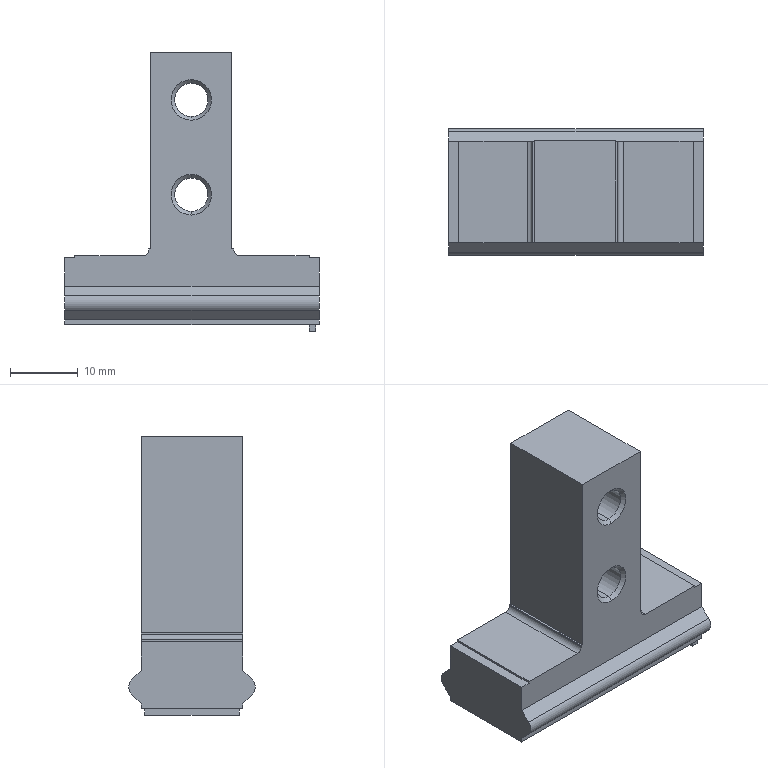Part | SolidWorks | features BaseBody 1 | 1 solid | 45 faces | box 37.6 x 18.7 x 41.2 mm | volume 11010 mm3 | plane 29 | cone 8 | cylinder 8 | commonest cylinder face diameters 4.917 x4 1.6 x2 3 x2
STEP:
#1=CARTESIAN_POINT('',(-30.,-6.958,35.659));
#2=VERTEX_POINT('',#1);
#3=CARTESIAN_POINT('',(-30.,-6.958,30.741));
#4=VERTEX_POINT('',#3);
#5=CARTESIAN_POINT('',(-30.,-6.958,33.2));
#6=DIRECTION('',(0.,-1.,0.));
#7=DIRECTION('',(0.,0.,-1.));
#8=AXIS2_PLACEMENT_3D('',#5,#6,#7);
#9=CIRCLE('',#8,2.459);
#10=EDGE_CURVE('',#2,#4,#9,.T.);
#11=ORIENTED_EDGE('',*,*,#10,.F.);
#12=CARTESIAN_POINT('',(-30.,-7.5,36.2));
#13=VERTEX_POINT('',#12);
#14=CARTESIAN_POINT('',(-30.,-6.958,35.659));
#15=DIRECTION('',(0.,-0.7071,0.7071));
#16=VECTOR('',#15,1000.);
#17=LINE('',#14,#16);
#18=EDGE_CURVE('',#2,#13,#17,.T.);
#19=ORIENTED_EDGE('',*,*,#18,.T.);
#20=CARTESIAN_POINT('',(-30.,-7.5,30.2));
#21=VERTEX_POINT('',#20);
#22=CARTESIAN_POINT('',(-30.,-7.5,33.2));
#23=DIRECTION('',(0.,-1.,0.));
#24=DIRECTION('',(0.,0.,-1.));
#25=AXIS2_PLACEMENT_3D('',#22,#23,#24);
#26=CIRCLE('',#25,3.);
#27=EDGE_CURVE('',#13,#21,#26,.T.);
#28=ORIENTED_EDGE('',*,*,#27,.T.);
#29=CARTESIAN_POINT('',(-30.,-6.958,30.741));
#30=DIRECTION('',(0.,-0.7071,-0.7071));
#31=VECTOR('',#30,1000.);
#32=LINE('',#29,#31);
#33=EDGE_CURVE('',#4,#21,#32,.T.);
#34=ORIENTED_EDGE('',*,*,#33,.F.);
#35=EDGE_LOOP('',(#11,#19,#28,#34));
#36=FACE_OUTER_BOUND('',#35,.T.);
#37=CARTESIAN_POINT('',(-30.,-6.958,33.2));
#38=DIRECTION('',(0.,-1.,0.));
#39=DIRECTION('',(0.,0.,-1.));
#40=AXIS2_PLACEMENT_3D('',#37,#38,#39);
#41=CONICAL_SURFACE('',#40,2.459,0.7854);
#42=ADVANCED_FACE('',(#36),#41,.F.);
#43=CARTESIAN_POINT('',(-30.,-6.958,21.659));
#44=VERTEX_POINT('',#43);
#45=CARTESIAN_POINT('',(-30.,-6.958,16.741));
#46=VERTEX_POINT('',#45);
#47=CARTESIAN_POINT('',(-30.,-6.958,19.2));
#48=DIRECTION('',(0.,-1.,0.));
#49=DIRECTION('',(0.,0.,-1.));
#50=AXIS2_PLACEMENT_3D('',#47,#48,#49);
#51=CIRCLE('',#50,2.459);
#52=EDGE_CURVE('',#44,#46,#51,.T.);
#53=ORIENTED_EDGE('',*,*,#52,.F.);
#54=CARTESIAN_POINT('',(-30.,-7.5,22.2));
#55=VERTEX_POINT('',#54);
#56=CARTESIAN_POINT('',(-30.,-6.958,21.658));
#57=DIRECTION('',(0.,-0.7071,0.7071));
#58=VECTOR('',#57,1000.);
#59=LINE('',#56,#58);
#60=EDGE_CURVE('',#44,#55,#59,.T.);
#61=ORIENTED_EDGE('',*,*,#60,.T.);
#62=CARTESIAN_POINT('',(-30.,-7.5,16.2));
#63=VERTEX_POINT('',#62);
#64=CARTESIAN_POINT('',(-30.,-7.5,19.2));
#65=DIRECTION('',(0.,-1.,0.));
#66=DIRECTION('',(0.,0.,-1.));
#67=AXIS2_PLACEMENT_3D('',#64,#65,#66);
#68=CIRCLE('',#67,3.);
#69=EDGE_CURVE('',#55,#63,#68,.T.);
#70=ORIENTED_EDGE('',*,*,#69,.T.);
#71=CARTESIAN_POINT('',(-30.,-6.958,16.741));
#72=DIRECTION('',(0.,-0.7071,-0.7071));
#73=VECTOR('',#72,1000.);
#74=LINE('',#71,#73);
#75=EDGE_CURVE('',#46,#63,#74,.T.);
#76=ORIENTED_EDGE('',*,*,#75,.F.);
#77=EDGE_LOOP('',(#53,#61,#70,#76));
#78=FACE_OUTER_BOUND('',#77,.T.);
#79=CARTESIAN_POINT('',(-30.,-6.958,19.2));
#80=DIRECTION('',(0.,-1.,0.));
#81=DIRECTION('',(0.,0.,-1.));
#82=AXIS2_PLACEMENT_3D('',#79,#80,#81);
#83=CONICAL_SURFACE('',#82,2.458,0.7854);
#84=ADVANCED_FACE('',(#78),#83,.F.);
#85=CARTESIAN_POINT('',(-30.,6.958,35.659));
#86=VERTEX_POINT('',#85);
#87=CARTESIAN_POINT('',(-30.,6.958,30.741));
#88=VERTEX_POINT('',#87);
#89=CARTESIAN_POINT('',(-30.,6.958,33.2));
#90=DIRECTION('',(0.,-1.,0.));
#91=DIRECTION('',(0.,0.,-1.));
#92=AXIS2_PLACEMENT_3D('',#89,#90,#91);
#93=CIRCLE('',#92,2.459);
#94=EDGE_CURVE('',#86,#88,#93,.T.);
#95=ORIENTED_EDGE('',*,*,#94,.F.);
#96=CARTESIAN_POINT('',(-30.,-7.5,35.659));
#97=DIRECTION('',(0.,-1.,0.));
#98=VECTOR('',#97,1000.);
#99=LINE('',#96,#98);
#100=EDGE_CURVE('',#86,#2,#99,.T.);
#101=ORIENTED_EDGE('',*,*,#100,.T.);
#102=ORIENTED_EDGE('',*,*,#10,.T.);
#103=CARTESIAN_POINT('',(-30.,-7.5,30.741));
#104=DIRECTION('',(0.,-1.,0.));
#105=VECTOR('',#104,1000.);
#106=LINE('',#103,#105);
#107=EDGE_CURVE('',#88,#4,#106,.T.);
#108=ORIENTED_EDGE('',*,*,#107,.F.);
#109=EDGE_LOOP('',(#95,#101,#102,#108));
#110=FACE_OUTER_BOUND('',#109,.T.);
#111=CARTESIAN_POINT('',(-30.,-7.5,33.2));
#112=DIRECTION('',(0.,-1.,0.));
#113=DIRECTION('',(0.,0.,-1.));
#114=AXIS2_PLACEMENT_3D('',#111,#112,#113);
#115=CYLINDRICAL_SURFACE('',#114,2.459);
#116=ADVANCED_FACE('',(#110),#115,.F.);
#117=CARTESIAN_POINT('',(-30.,6.958,21.659));
#118=VERTEX_POINT('',#117);
#119=CARTESIAN_POINT('',(-30.,6.958,16.741));
#120=VERTEX_POINT('',#119);
#121=CARTESIAN_POINT('',(-30.,6.958,19.2));
#122=DIRECTION('',(0.,-1.,0.));
#123=DIRECTION('',(0.,0.,-1.));
#124=AXIS2_PLACEMENT_3D('',#121,#122,#123);
#125=CIRCLE('',#124,2.459);
#126=EDGE_CURVE('',#118,#120,#125,.T.);
#127=ORIENTED_EDGE('',*,*,#126,.F.);
#128=CARTESIAN_POINT('',(-30.,-7.5,21.658));
#129=DIRECTION('',(0.,-1.,0.));
#130=VECTOR('',#129,1000.);
#131=LINE('',#128,#130);
#132=EDGE_CURVE('',#118,#44,#131,.T.);
#133=ORIENTED_EDGE('',*,*,#132,.T.);
#134=ORIENTED_EDGE('',*,*,#52,.T.);
#135=CARTESIAN_POINT('',(-30.,-7.5,16.741));
#136=DIRECTION('',(0.,-1.,0.));
#137=VECTOR('',#136,1000.);
#138=LINE('',#135,#137);
#139=EDGE_CURVE('',#120,#46,#138,.T.);
#140=ORIENTED_EDGE('',*,*,#139,.F.);
#141=EDGE_LOOP('',(#127,#133,#134,#140));
#142=FACE_OUTER_BOUND('',#141,.T.);
#143=CARTESIAN_POINT('',(-30.,-7.5,19.2));
#144=DIRECTION('',(0.,-1.,0.));
#145=DIRECTION('',(0.,0.,-1.));
#146=AXIS2_PLACEMENT_3D('',#143,#144,#145);
#147=CYLINDRICAL_SURFACE('',#146,2.458);
#148=ADVANCED_FACE('',(#142),#147,.F.);
#149=ORIENTED_EDGE('',*,*,#94,.T.);
#150=CARTESIAN_POINT('',(-30.,7.5,30.2));
#151=VERTEX_POINT('',#150);
#152=CARTESIAN_POINT('',(-30.,7.5,30.2));
#153=DIRECTION('',(0.,0.7071,-0.7071));
#154=VECTOR('',#153,1000.);
#155=LINE('',#152,#154);
#156=EDGE_CURVE('',#88,#151,#155,.T.);
#157=ORIENTED_EDGE('',*,*,#156,.T.);
#158=CARTESIAN_POINT('',(-30.,7.5,36.2));
#159=VERTEX_POINT('',#158);
#160=CARTESIAN_POINT('',(-30.,7.5,33.2));
#161=DIRECTION('',(0.,-1.,0.));
#162=DIRECTION('',(0.,0.,-1.));
#163=AXIS2_PLACEMENT_3D('',#160,#161,#162);
#164=CIRCLE('',#163,3.);
#165=EDGE_CURVE('',#159,#151,#164,.T.);
#166=ORIENTED_EDGE('',*,*,#165,.F.);
#167=CARTESIAN_POINT('',(-30.,7.5,36.2));
#168=DIRECTION('',(0.,0.7071,0.7071));
#169=VECTOR('',#168,1000.);
#170=LINE('',#167,#169);
#171=EDGE_CURVE('',#86,#159,#170,.T.);
#172=ORIENTED_EDGE('',*,*,#171,.F.);
#173=EDGE_LOOP('',(#149,#157,#166,#172));
#174=FACE_OUTER_BOUND('',#173,.T.);
#175=CARTESIAN_POINT('',(-30.,7.5,33.2));
#176=DIRECTION('',(0.,1.,0.));
#177=DIRECTION('',(0.,0.,1.));
#178=AXIS2_PLACEMENT_3D('',#175,#176,#177);
#179=CONICAL_SURFACE('',#178,3.,0.7854);
#180=ADVANCED_FACE('',(#174),#179,.F.);
#181=ORIENTED_EDGE('',*,*,#126,.T.);
#182=CARTESIAN_POINT('',(-30.,7.5,16.2));
#183=VERTEX_POINT('',#182);
#184=CARTESIAN_POINT('',(-30.,7.5,16.2));
#185=DIRECTION('',(0.,0.7071,-0.7071));
#186=VECTOR('',#185,1000.);
#187=LINE('',#184,#186);
#188=EDGE_CURVE('',#120,#183,#187,.T.);
#189=ORIENTED_EDGE('',*,*,#188,.T.);
#190=CARTESIAN_POINT('',(-30.,7.5,22.2));
#191=VERTEX_POINT('',#190);
#192=CARTESIAN_POINT('',(-30.,7.5,19.2));
#193=DIRECTION('',(0.,-1.,0.));
#194=DIRECTION('',(0.,0.,-1.));
#195=AXIS2_PLACEMENT_3D('',#192,#193,#194);
#196=CIRCLE('',#195,3.);
#197=EDGE_CURVE('',#191,#183,#196,.T.);
#198=ORIENTED_EDGE('',*,*,#197,.F.);
#199=CARTESIAN_POINT('',(-30.,7.5,22.2));
#200=DIRECTION('',(0.,0.7071,0.7071));
#201=VECTOR('',#200,1000.);
#202=LINE('',#199,#201);
#203=EDGE_CURVE('',#118,#191,#202,.T.);
#204=ORIENTED_EDGE('',*,*,#203,.F.);
#205=EDGE_LOOP('',(#181,#189,#198,#204));
#206=FACE_OUTER_BOUND('',#205,.T.);
#207=CARTESIAN_POINT('',(-30.,7.5,19.2));
#208=DIRECTION('',(0.,1.,0.));
#209=DIRECTION('',(0.,0.,1.));
#210=AXIS2_PLACEMENT_3D('',#207,#208,#209);
#211=CONICAL_SURFACE('',#210,3.,0.7854);
#212=ADVANCED_FACE('',(#206),#211,.F.);
#213=CARTESIAN_POINT('',(-47.2,7.5,9.9));
#214=VERTEX_POINT('',#213);
#215=CARTESIAN_POINT('',(-48.7,7.5,9.9));
#216=VERTEX_POINT('',#215);
#217=CARTESIAN_POINT('',(-47.2,7.5,9.9));
#218=DIRECTION('',(-1.,0.,0.));
#219=VECTOR('',#218,1000.);
#220=LINE('',#217,#219);
#221=EDGE_CURVE('',#214,#216,#220,.T.);
#222=ORIENTED_EDGE('',*,*,#221,.F.);
#223=CARTESIAN_POINT('',(-47.2,7.5,10.2));
#224=VERTEX_POINT('',#223);
#225=CARTESIAN_POINT('',(-47.2,7.5,9.9));
#226=DIRECTION('',(0.,0.,1.));
#227=VECTOR('',#226,1000.);
#228=LINE('',#225,#227);
#229=EDGE_CURVE('',#214,#224,#228,.T.);
#230=ORIENTED_EDGE('',*,*,#229,.T.);
#231=CARTESIAN_POINT('',(-37.1,7.5,10.2));
#232=VERTEX_POINT('',#231);
#233=CARTESIAN_POINT('',(-47.2,7.5,10.2));
#234=DIRECTION('',(1.,0.,0.));
#235=VECTOR('',#234,1000.);
#236=LINE('',#233,#235);
#237=EDGE_CURVE('',#224,#232,#236,.T.);
#238=ORIENTED_EDGE('',*,*,#237,.T.);
#239=CARTESIAN_POINT('',(-36.3,7.5,11.));
#240=VERTEX_POINT('',#239);
#241=CARTESIAN_POINT('',(-37.1,7.5,11.));
#242=DIRECTION('',(0.,1.,0.));
#243=DIRECTION('',(1.,0.,0.));
#244=AXIS2_PLACEMENT_3D('',#241,#242,#243);
#245=CIRCLE('',#244,0.8);
#246=EDGE_CURVE('',#240,#232,#245,.T.);
#247=ORIENTED_EDGE('',*,*,#246,.F.);
#248=CARTESIAN_POINT('',(-36.3,7.5,11.2));
#249=VERTEX_POINT('',#248);
#250=CARTESIAN_POINT('',(-36.3,7.5,11.));
#251=DIRECTION('',(0.,0.,1.));
#252=VECTOR('',#251,1000.);
#253=LINE('',#250,#252);
#254=EDGE_CURVE('',#240,#249,#253,.T.);
#255=ORIENTED_EDGE('',*,*,#254,.T.);
#256=CARTESIAN_POINT('',(-36.,7.5,11.2));
#257=VERTEX_POINT('',#256);
#258=CARTESIAN_POINT('',(-36.3,7.5,11.2));
#259=DIRECTION('',(1.,0.,0.));
#260=VECTOR('',#259,1000.);
#261=LINE('',#258,#260);
#262=EDGE_CURVE('',#249,#257,#261,.T.);
#263=ORIENTED_EDGE('',*,*,#262,.T.);
#264=CARTESIAN_POINT('',(-36.,7.5,40.2));
#265=VERTEX_POINT('',#264);
#266=CARTESIAN_POINT('',(-36.,7.5,11.2));
#267=DIRECTION('',(0.,0.,1.));
#268=VECTOR('',#267,1000.);
#269=LINE('',#266,#268);
#270=EDGE_CURVE('',#257,#265,#269,.T.);
#271=ORIENTED_EDGE('',*,*,#270,.T.);
#272=CARTESIAN_POINT('',(-24.,7.5,40.2));
#273=VERTEX_POINT('',#272);
#274=CARTESIAN_POINT('',(-36.,7.5,40.2));
#275=DIRECTION('',(1.,0.,0.));
#276=VECTOR('',#275,1000.);
#277=LINE('',#274,#276);
#278=EDGE_CURVE('',#265,#273,#277,.T.);
#279=ORIENTED_EDGE('',*,*,#278,.T.);
#280=CARTESIAN_POINT('',(-24.,7.5,11.2));
#281=VERTEX_POINT('',#280);
#282=CARTESIAN_POINT('',(-24.,7.5,40.2));
#283=DIRECTION('',(0.,0.,-1.));
#284=VECTOR('',#283,1000.);
#285=LINE('',#282,#284);
#286=EDGE_CURVE('',#273,#281,#285,.T.);
#287=ORIENTED_EDGE('',*,*,#286,.T.);
#288=CARTESIAN_POINT('',(-23.7,7.5,11.2));
#289=VERTEX_POINT('',#288);
#290=CARTESIAN_POINT('',(-24.,7.5,11.2));
#291=DIRECTION('',(1.,0.,0.));
#292=VECTOR('',#291,1000.);
#293=LINE('',#290,#292);
#294=EDGE_CURVE('',#281,#289,#293,.T.);
#295=ORIENTED_EDGE('',*,*,#294,.T.);
#296=CARTESIAN_POINT('',(-23.7,7.5,11.));
#297=VERTEX_POINT('',#296);
#298=CARTESIAN_POINT('',(-23.7,7.5,11.2));
#299=DIRECTION('',(0.,0.,-1.));
#300=VECTOR('',#299,1000.);
#301=LINE('',#298,#300);
#302=EDGE_CURVE('',#289,#297,#301,.T.);
#303=ORIENTED_EDGE('',*,*,#302,.T.);
#304=CARTESIAN_POINT('',(-22.9,7.5,10.2));
#305=VERTEX_POINT('',#304);
#306=CARTESIAN_POINT('',(-22.9,7.5,11.));
#307=DIRECTION('',(0.,1.,0.));
#308=DIRECTION('',(0.,0.,-1.));
#309=AXIS2_PLACEMENT_3D('',#306,#307,#308);
#310=CIRCLE('',#309,0.8);
#311=EDGE_CURVE('',#305,#297,#310,.T.);
#312=ORIENTED_EDGE('',*,*,#311,.F.);
#313=CARTESIAN_POINT('',(-12.6,7.5,10.2));
#314=VERTEX_POINT('',#313);
#315=CARTESIAN_POINT('',(-22.9,7.5,10.2));
#316=DIRECTION('',(1.,0.,0.));
#317=VECTOR('',#316,1000.);
#318=LINE('',#315,#317);
#319=EDGE_CURVE('',#305,#314,#318,.T.);
#320=ORIENTED_EDGE('',*,*,#319,.T.);
#321=CARTESIAN_POINT('',(-12.6,7.5,9.9));
#322=VERTEX_POINT('',#321);
#323=CARTESIAN_POINT('',(-12.6,7.5,10.2));
#324=DIRECTION('',(0.,0.,-1.));
#325=VECTOR('',#324,1000.);
#326=LINE('',#323,#325);
#327=EDGE_CURVE('',#314,#322,#326,.T.);
#328=ORIENTED_EDGE('',*,*,#327,.T.);
#329=CARTESIAN_POINT('',(-11.1,7.5,9.9));
#330=VERTEX_POINT('',#329);
#331=CARTESIAN_POINT('',(-11.1,7.5,9.9));
#332=DIRECTION('',(-1.,0.,0.));
#333=VECTOR('',#332,1000.);
#334=LINE('',#331,#333);
#335=EDGE_CURVE('',#330,#322,#334,.T.);
#336=ORIENTED_EDGE('',*,*,#335,.F.);
#337=CARTESIAN_POINT('',(-11.1,7.5,5.672));
#338=VERTEX_POINT('',#337);
#339=CARTESIAN_POINT('',(-11.1,7.5,5.672));
#340=DIRECTION('',(0.,0.,1.));
#341=VECTOR('',#340,1000.);
#342=LINE('',#339,#341);
#343=EDGE_CURVE('',#338,#330,#342,.T.);
#344=ORIENTED_EDGE('',*,*,#343,.F.);
#345=CARTESIAN_POINT('',(-48.7,7.5,5.672));
#346=VERTEX_POINT('',#345);
#347=CARTESIAN_POINT('',(-11.1,7.5,5.672));
#348=DIRECTION('',(-1.,0.,0.));
#349=VECTOR('',#348,1000.);
#350=LINE('',#347,#349);
#351=EDGE_CURVE('',#338,#346,#350,.T.);
#352=ORIENTED_EDGE('',*,*,#351,.T.);
#353=CARTESIAN_POINT('',(-48.7,7.5,5.672));
#354=DIRECTION('',(0.,0.,1.));
#355=VECTOR('',#354,1000.);
#356=LINE('',#353,#355);
#357=EDGE_CURVE('',#346,#216,#356,.T.);
#358=ORIENTED_EDGE('',*,*,#357,.T.);
#359=EDGE_LOOP('',(#222,#230,#238,#247,#255,#263,#271,#279,#287,#295,#303,#312,#320,#328,#336,#344,#352,#358));
#360=FACE_OUTER_BOUND('',#359,.T.);
#361=ORIENTED_EDGE('',*,*,#197,.T.);
#362=CARTESIAN_POINT('',(-30.,7.5,19.2));
#363=DIRECTION('',(0.,-1.,0.));
#364=DIRECTION('',(0.,0.,-1.));
#365=AXIS2_PLACEMENT_3D('',#362,#363,#364);
#366=CIRCLE('',#365,3.);
#367=EDGE_CURVE('',#183,#191,#366,.T.);
#368=ORIENTED_EDGE('',*,*,#367,.T.);
#369=EDGE_LOOP('',(#361,#368));
#370=FACE_BOUND('',#369,.T.);
#371=ORIENTED_EDGE('',*,*,#165,.T.);
#372=CARTESIAN_POINT('',(-30.,7.5,33.2));
#373=DIRECTION('',(0.,-1.,0.));
#374=DIRECTION('',(0.,0.,-1.));
#375=AXIS2_PLACEMENT_3D('',#372,#373,#374);
#376=CIRCLE('',#375,3.);
#377=EDGE_CURVE('',#151,#159,#376,.T.);
#378=ORIENTED_EDGE('',*,*,#377,.T.);
#379=EDGE_LOOP('',(#371,#378));
#380=FACE_BOUND('',#379,.T.);
#381=CARTESIAN_POINT('',(-37.1,7.5,11.));
#382=DIRECTION('',(0.,1.,0.));
#383=DIRECTION('',(0.,0.,1.));
#384=AXIS2_PLACEMENT_3D('',#381,#382,#383);
#385=PLANE('',#384);
#386=ADVANCED_FACE('',(#360,#370,#380),#385,.T.);
#387=CARTESIAN_POINT('',(-47.2,-7.5,9.9));
#388=VERTEX_POINT('',#387);
#389=CARTESIAN_POINT('',(-47.2,7.5,9.9));
#390=DIRECTION('',(0.,-1.,0.));
#391=VECTOR('',#390,1000.);
#392=LINE('',#389,#391);
#393=EDGE_CURVE('',#214,#388,#392,.T.);
#394=ORIENTED_EDGE('',*,*,#393,.F.);
#395=ORIENTED_EDGE('',*,*,#221,.T.);
#396=CARTESIAN_POINT('',(-48.7,-7.5,9.9));
#397=VERTEX_POINT('',#396);
#398=CARTESIAN_POINT('',(-48.7,7.5,9.9));
#399=DIRECTION('',(0.,-1.,0.));
#400=VECTOR('',#399,1000.);
#401=LINE('',#398,#400);
#402=EDGE_CURVE('',#216,#397,#401,.T.);
#403=ORIENTED_EDGE('',*,*,#402,.T.);
#404=CARTESIAN_POINT('',(-47.2,-7.5,9.9));
#405=DIRECTION('',(-1.,0.,0.));
#406=VECTOR('',#405,1000.);
#407=LINE('',#404,#406);
#408=EDGE_CURVE('',#388,#397,#407,.T.);
#409=ORIENTED_EDGE('',*,*,#408,.F.);
#410=EDGE_LOOP('',(#394,#395,#403,#409));
#411=FACE_OUTER_BOUND('',#410,.T.);
#412=CARTESIAN_POINT('',(-11.1,7.5,9.9));
#413=DIRECTION('',(0.,0.,-1.));
#414=DIRECTION('',(-1.,0.,0.));
#415=AXIS2_PLACEMENT_3D('',#412,#413,#414);
#416=PLANE('',#415);
#417=ADVANCED_FACE('',(#411),#416,.F.);
#418=ORIENTED_EDGE('',*,*,#229,.F.);
#419=ORIENTED_EDGE('',*,*,#393,.T.);
#420=CARTESIAN_POINT('',(-47.2,-7.5,10.2));
#421=VERTEX_POINT('',#420);
#422=CARTESIAN_POINT('',(-47.2,-7.5,9.9));
#423=DIRECTION('',(0.,0.,1.));
#424=VECTOR('',#423,1000.);
#425=LINE('',#422,#424);
#426=EDGE_CURVE('',#388,#421,#425,.T.);
#427=ORIENTED_EDGE('',*,*,#426,.T.);
#428=CARTESIAN_POINT('',(-47.2,-7.5,10.2));
#429=DIRECTION('',(0.,1.,0.));
#430=VECTOR('',#429,1000.);
#431=LINE('',#428,#430);
#432=EDGE_CURVE('',#421,#224,#431,.T.);
#433=ORIENTED_EDGE('',*,*,#432,.T.);
#434=EDGE_LOOP('',(#418,#419,#427,#433));
#435=FACE_OUTER_BOUND('',#434,.T.);
#436=CARTESIAN_POINT('',(-47.2,50.,30.));
#437=DIRECTION('',(-1.,0.,0.));
#438=DIRECTION('',(0.,0.,1.));
#439=AXIS2_PLACEMENT_3D('',#436,#437,#438);
#440=PLANE('',#439);
#441=ADVANCED_FACE('',(#435),#440,.T.);
#442=ORIENTED_EDGE('',*,*,#432,.F.);
#443=CARTESIAN_POINT('',(-37.1,-7.5,10.2));
#444=VERTEX_POINT('',#443);
#445=CARTESIAN_POINT('',(-47.2,-7.5,10.2));
#446=DIRECTION('',(1.,0.,0.));
#447=VECTOR('',#446,1000.);
#448=LINE('',#445,#447);
#449=EDGE_CURVE('',#421,#444,#448,.T.);
#450=ORIENTED_EDGE('',*,*,#449,.T.);
#451=CARTESIAN_POINT('',(-37.1,7.5,10.2));
#452=DIRECTION('',(0.,-1.,0.));
#453=VECTOR('',#452,1000.);
#454=LINE('',#451,#453);
#455=EDGE_CURVE('',#232,#444,#454,.T.);
#456=ORIENTED_EDGE('',*,*,#455,.F.);
#457=ORIENTED_EDGE('',*,*,#237,.F.);
#458=EDGE_LOOP('',(#442,#450,#456,#457));
#459=FACE_OUTER_BOUND('',#458,.T.);
#460=CARTESIAN_POINT('',(-48.7,7.5,10.2));
#461=DIRECTION('',(0.,0.,-1.));
#462=DIRECTION('',(-1.,0.,0.));
#463=AXIS2_PLACEMENT_3D('',#460,#461,#462);
#464=PLANE('',#463);
#465=ADVANCED_FACE('',(#459),#464,.F.);
#466=CARTESIAN_POINT('',(-36.3,-7.5,11.));
#467=VERTEX_POINT('',#466);
#468=CARTESIAN_POINT('',(-37.1,-7.5,11.));
#469=DIRECTION('',(0.,1.,0.));
#470=DIRECTION('',(1.,0.,0.));
#471=AXIS2_PLACEMENT_3D('',#468,#469,#470);
#472=CIRCLE('',#471,0.8);
#473=EDGE_CURVE('',#467,#444,#472,.T.);
#474=ORIENTED_EDGE('',*,*,#473,.F.);
#475=CARTESIAN_POINT('',(-36.3,7.5,11.));
#476=DIRECTION('',(0.,-1.,0.));
#477=VECTOR('',#476,1000.);
#478=LINE('',#475,#477);
#479=EDGE_CURVE('',#240,#467,#478,.T.);
#480=ORIENTED_EDGE('',*,*,#479,.F.);
#481=ORIENTED_EDGE('',*,*,#246,.T.);
#482=ORIENTED_EDGE('',*,*,#455,.T.);
#483=EDGE_LOOP('',(#474,#480,#481,#482));
#484=FACE_OUTER_BOUND('',#483,.T.);
#485=CARTESIAN_POINT('',(-37.1,7.5,11.));
#486=DIRECTION('',(0.,-1.,0.));
#487=DIRECTION('',(0.,0.,-1.));
#488=AXIS2_PLACEMENT_3D('',#485,#486,#487);
#489=CYLINDRICAL_SURFACE('',#488,0.8);
#490=ADVANCED_FACE('',(#484),#489,.F.);
#491=CARTESIAN_POINT('',(-36.3,-7.5,11.2));
#492=VERTEX_POINT('',#491);
#493=CARTESIAN_POINT('',(-36.3,-7.5,11.));
#494=DIRECTION('',(0.,0.,1.));
#495=VECTOR('',#494,1000.);
#496=LINE('',#493,#495);
#497=EDGE_CURVE('',#467,#492,#496,.T.);
#498=ORIENTED_EDGE('',*,*,#497,.T.);
#499=CARTESIAN_POINT('',(-36.3,7.5,11.2));
#500=DIRECTION('',(0.,-1.,0.));
#501=VECTOR('',#500,1000.);
#502=LINE('',#499,#501);
#503=EDGE_CURVE('',#249,#492,#502,.T.);
#504=ORIENTED_EDGE('',*,*,#503,.F.);
#505=ORIENTED_EDGE('',*,*,#254,.F.);
#506=ORIENTED_EDGE('',*,*,#479,.T.);
#507=EDGE_LOOP('',(#498,#504,#505,#506));
#508=FACE_OUTER_BOUND('',#507,.T.);
#509=CARTESIAN_POINT('',(-36.3,7.5,11.));
#510=DIRECTION('',(1.,0.,0.));
#511=DIRECTION('',(0.,0.,-1.));
#512=AXIS2_PLACEMENT_3D('',#509,#510,#511);
#513=PLANE('',#512);
#514=ADVANCED_FACE('',(#508),#513,.F.);
#515=CARTESIAN_POINT('',(-36.,-7.5,11.2));
#516=VERTEX_POINT('',#515);
#517=CARTESIAN_POINT('',(-36.3,-7.5,11.2));
#518=DIRECTION('',(1.,0.,0.));
#519=VECTOR('',#518,1000.);
#520=LINE('',#517,#519);
#521=EDGE_CURVE('',#492,#516,#520,.T.);
#522=ORIENTED_EDGE('',*,*,#521,.T.);
#523=CARTESIAN_POINT('',(-36.,7.5,11.2));
#524=DIRECTION('',(0.,-1.,0.));
#525=VECTOR('',#524,1000.);
#526=LINE('',#523,#525);
#527=EDGE_CURVE('',#257,#516,#526,.T.);
#528=ORIENTED_EDGE('',*,*,#527,.F.);
#529=ORIENTED_EDGE('',*,*,#262,.F.);
#530=ORIENTED_EDGE('',*,*,#503,.T.);
#531=EDGE_LOOP('',(#522,#528,#529,#530));
#532=FACE_OUTER_BOUND('',#531,.T.);
#533=CARTESIAN_POINT('',(-36.3,7.5,11.2));
#534=DIRECTION('',(0.,0.,-1.));
#535=DIRECTION('',(-1.,0.,0.));
#536=AXIS2_PLACEMENT_3D('',#533,#534,#535);
#537=PLANE('',#536);
#538=ADVANCED_FACE('',(#532),#537,.F.);
#539=CARTESIAN_POINT('',(-36.,-7.5,40.2));
#540=VERTEX_POINT('',#539);
#541=CARTESIAN_POINT('',(-36.,-7.5,11.2));
#542=DIRECTION('',(0.,0.,1.));
#543=VECTOR('',#542,1000.);
#544=LINE('',#541,#543);
#545=EDGE_CURVE('',#516,#540,#544,.T.);
#546=ORIENTED_EDGE('',*,*,#545,.T.);
#547=CARTESIAN_POINT('',(-36.,7.5,40.2));
#548=DIRECTION('',(0.,-1.,0.));
#549=VECTOR('',#548,1000.);
#550=LINE('',#547,#549);
#551=EDGE_CURVE('',#265,#540,#550,.T.);
#552=ORIENTED_EDGE('',*,*,#551,.F.);
#553=ORIENTED_EDGE('',*,*,#270,.F.);
#554=ORIENTED_EDGE('',*,*,#527,.T.);
#555=EDGE_LOOP('',(#546,#552,#553,#554));
#556=FACE_OUTER_BOUND('',#555,.T.);
#557=CARTESIAN_POINT('',(-36.,7.5,11.2));
#558=DIRECTION('',(1.,0.,0.));
#559=DIRECTION('',(0.,0.,-1.));
#560=AXIS2_PLACEMENT_3D('',#557,#558,#559);
#561=PLANE('',#560);
#562=ADVANCED_FACE('',(#556),#561,.F.);
#563=CARTESIAN_POINT('',(-24.,-7.5,40.2));
#564=VERTEX_POINT('',#563);
#565=CARTESIAN_POINT('',(-36.,-7.5,40.2));
#566=DIRECTION('',(1.,0.,0.));
#567=VECTOR('',#566,1000.);
#568=LINE('',#565,#567);
#569=EDGE_CURVE('',#540,#564,#568,.T.);
#570=ORIENTED_EDGE('',*,*,#569,.T.);
#571=CARTESIAN_POINT('',(-24.,7.5,40.2));
#572=DIRECTION('',(0.,-1.,0.));
#573=VECTOR('',#572,1000.);
#574=LINE('',#571,#573);
#575=EDGE_CURVE('',#273,#564,#574,.T.);
#576=ORIENTED_EDGE('',*,*,#575,.F.);
#577=ORIENTED_EDGE('',*,*,#278,.F.);
#578=ORIENTED_EDGE('',*,*,#551,.T.);
#579=EDGE_LOOP('',(#570,#576,#577,#578));
#580=FACE_OUTER_BOUND('',#579,.T.);
#581=CARTESIAN_POINT('',(-36.,7.5,40.2));
#582=DIRECTION('',(0.,0.,-1.));
#583=DIRECTION('',(-1.,0.,0.));
#584=AXIS2_PLACEMENT_3D('',#581,#582,#583);
#585=PLANE('',#584);
#586=ADVANCED_FACE('',(#580),#585,.F.);
#587=CARTESIAN_POINT('',(-24.,-7.5,11.2));
#588=VERTEX_POINT('',#587);
#589=CARTESIAN_POINT('',(-24.,-7.5,40.2));
#590=DIRECTION('',(0.,0.,-1.));
#591=VECTOR('',#590,1000.);
#592=LINE('',#589,#591);
#593=EDGE_CURVE('',#564,#588,#592,.T.);
#594=ORIENTED_EDGE('',*,*,#593,.T.);
#595=CARTESIAN_POINT('',(-24.,7.5,11.2));
#596=DIRECTION('',(0.,-1.,0.));
#597=VECTOR('',#596,1000.);
#598=LINE('',#595,#597);
#599=EDGE_CURVE('',#281,#588,#598,.T.);
#600=ORIENTED_EDGE('',*,*,#599,.F.);
#601=ORIENTED_EDGE('',*,*,#286,.F.);
#602=ORIENTED_EDGE('',*,*,#575,.T.);
#603=EDGE_LOOP('',(#594,#600,#601,#602));
#604=FACE_OUTER_BOUND('',#603,.T.);
#605=CARTESIAN_POINT('',(-24.,7.5,40.2));
#606=DIRECTION('',(-1.,0.,0.));
#607=DIRECTION('',(0.,0.,1.));
#608=AXIS2_PLACEMENT_3D('',#605,#606,#607);
#609=PLANE('',#608);
#610=ADVANCED_FACE('',(#604),#609,.F.);
#611=CARTESIAN_POINT('',(-23.7,-7.5,11.2));
#612=VERTEX_POINT('',#611);
#613=CARTESIAN_POINT('',(-24.,-7.5,11.2));
#614=DIRECTION('',(1.,0.,0.));
#615=VECTOR('',#614,1000.);
#616=LINE('',#613,#615);
#617=EDGE_CURVE('',#588,#612,#616,.T.);
#618=ORIENTED_EDGE('',*,*,#617,.T.);
#619=CARTESIAN_POINT('',(-23.7,7.5,11.2));
#620=DIRECTION('',(0.,-1.,0.));
#621=VECTOR('',#620,1000.);
#622=LINE('',#619,#621);
#623=EDGE_CURVE('',#289,#612,#622,.T.);
#624=ORIENTED_EDGE('',*,*,#623,.F.);
#625=ORIENTED_EDGE('',*,*,#294,.F.);
#626=ORIENTED_EDGE('',*,*,#599,.T.);
#627=EDGE_LOOP('',(#618,#624,#625,#626));
#628=FACE_OUTER_BOUND('',#627,.T.);
#629=CARTESIAN_POINT('',(-24.,7.5,11.2));
#630=DIRECTION('',(0.,0.,-1.));
#631=DIRECTION('',(-1.,0.,0.));
#632=AXIS2_PLACEMENT_3D('',#629,#630,#631);
#633=PLANE('',#632);
#634=ADVANCED_FACE('',(#628),#633,.F.);
#635=CARTESIAN_POINT('',(-23.7,-7.5,11.));
#636=VERTEX_POINT('',#635);
#637=CARTESIAN_POINT('',(-23.7,-7.5,11.2));
#638=DIRECTION('',(0.,0.,-1.));
#639=VECTOR('',#638,1000.);
#640=LINE('',#637,#639);
#641=EDGE_CURVE('',#612,#636,#640,.T.);
#642=ORIENTED_EDGE('',*,*,#641,.T.);
#643=CARTESIAN_POINT('',(-23.7,7.5,11.));
#644=DIRECTION('',(0.,-1.,0.));
#645=VECTOR('',#644,1000.);
#646=LINE('',#643,#645);
#647=EDGE_CURVE('',#297,#636,#646,.T.);
#648=ORIENTED_EDGE('',*,*,#647,.F.);
#649=ORIENTED_EDGE('',*,*,#302,.F.);
#650=ORIENTED_EDGE('',*,*,#623,.T.);
#651=EDGE_LOOP('',(#642,#648,#649,#650));
#652=FACE_OUTER_BOUND('',#651,.T.);
#653=CARTESIAN_POINT('',(-23.7,7.5,11.2));
#654=DIRECTION('',(-1.,0.,0.));
#655=DIRECTION('',(0.,0.,1.));
#656=AXIS2_PLACEMENT_3D('',#653,#654,#655);
#657=PLANE('',#656);
#658=ADVANCED_FACE('',(#652),#657,.F.);
#659=CARTESIAN_POINT('',(-22.9,-7.5,10.2));
#660=VERTEX_POINT('',#659);
#661=CARTESIAN_POINT('',(-22.9,-7.5,11.));
#662=DIRECTION('',(0.,1.,0.));
#663=DIRECTION('',(0.,0.,-1.));
#664=AXIS2_PLACEMENT_3D('',#661,#662,#663);
#665=CIRCLE('',#664,0.8);
#666=EDGE_CURVE('',#660,#636,#665,.T.);
#667=ORIENTED_EDGE('',*,*,#666,.F.);
#668=CARTESIAN_POINT('',(-22.9,7.5,10.2));
#669=DIRECTION('',(0.,-1.,0.));
#670=VECTOR('',#669,1000.);
#671=LINE('',#668,#670);
#672=EDGE_CURVE('',#305,#660,#671,.T.);
#673=ORIENTED_EDGE('',*,*,#672,.F.);
#674=ORIENTED_EDGE('',*,*,#311,.T.);
#675=ORIENTED_EDGE('',*,*,#647,.T.);
#676=EDGE_LOOP('',(#667,#673,#674,#675));
#677=FACE_OUTER_BOUND('',#676,.T.);
#678=CARTESIAN_POINT('',(-22.9,7.5,11.));
#679=DIRECTION('',(0.,-1.,0.));
#680=DIRECTION('',(0.,0.,-1.));
#681=AXIS2_PLACEMENT_3D('',#678,#679,#680);
#682=CYLINDRICAL_SURFACE('',#681,0.8);
#683=ADVANCED_FACE('',(#677),#682,.F.);
#684=CARTESIAN_POINT('',(-12.6,-7.5,10.2));
#685=VERTEX_POINT('',#684);
#686=CARTESIAN_POINT('',(-12.6,7.5,10.2));
#687=DIRECTION('',(0.,-1.,0.));
#688=VECTOR('',#687,1000.);
#689=LINE('',#686,#688);
#690=EDGE_CURVE('',#314,#685,#689,.T.);
#691=ORIENTED_EDGE('',*,*,#690,.F.);
#692=ORIENTED_EDGE('',*,*,#319,.F.);
#693=ORIENTED_EDGE('',*,*,#672,.T.);
#694=CARTESIAN_POINT('',(-22.9,-7.5,10.2));
#695=DIRECTION('',(1.,0.,0.));
#696=VECTOR('',#695,1000.);
#697=LINE('',#694,#696);
#698=EDGE_CURVE('',#660,#685,#697,.T.);
#699=ORIENTED_EDGE('',*,*,#698,.T.);
#700=EDGE_LOOP('',(#691,#692,#693,#699));
#701=FACE_OUTER_BOUND('',#700,.T.);
#702=CARTESIAN_POINT('',(-22.9,7.5,10.2));
#703=DIRECTION('',(0.,0.,-1.));
#704=DIRECTION('',(-1.,0.,0.));
#705=AXIS2_PLACEMENT_3D('',#702,#703,#704);
#706=PLANE('',#705);
#707=ADVANCED_FACE('',(#701),#706,.F.);
#708=CARTESIAN_POINT('',(-12.6,-7.5,9.9));
#709=VERTEX_POINT('',#708);
#710=CARTESIAN_POINT('',(-12.6,-7.5,10.2));
#711=DIRECTION('',(0.,0.,-1.));
#712=VECTOR('',#711,1000.);
#713=LINE('',#710,#712);
#714=EDGE_CURVE('',#685,#709,#713,.T.);
#715=ORIENTED_EDGE('',*,*,#714,.T.);
#716=CARTESIAN_POINT('',(-12.6,-7.5,9.9));
#717=DIRECTION('',(0.,1.,0.));
#718=VECTOR('',#717,1000.);
#719=LINE('',#716,#718);
#720=EDGE_CURVE('',#709,#322,#719,.T.);
#721=ORIENTED_EDGE('',*,*,#720,.T.);
#722=ORIENTED_EDGE('',*,*,#327,.F.);
#723=ORIENTED_EDGE('',*,*,#690,.T.);
#724=EDGE_LOOP('',(#715,#721,#722,#723));
#725=FACE_OUTER_BOUND('',#724,.T.);
#726=CARTESIAN_POINT('',(-12.6,50.,0.));
#727=DIRECTION('',(1.,0.,0.));
#728=DIRECTION('',(0.,0.,-1.));
#729=AXIS2_PLACEMENT_3D('',#726,#727,#728);
#730=PLANE('',#729);
#731=ADVANCED_FACE('',(#725),#730,.T.);
#732=ORIENTED_EDGE('',*,*,#720,.F.);
#733=CARTESIAN_POINT('',(-11.1,-7.5,9.9));
#734=VERTEX_POINT('',#733);
#735=CARTESIAN_POINT('',(-11.1,-7.5,9.9));
#736=DIRECTION('',(-1.,0.,0.));
#737=VECTOR('',#736,1000.);
#738=LINE('',#735,#737);
#739=EDGE_CURVE('',#734,#709,#738,.T.);
#740=ORIENTED_EDGE('',*,*,#739,.F.);
#741=CARTESIAN_POINT('',(-11.1,7.5,9.9));
#742=DIRECTION('',(0.,-1.,0.));
#743=VECTOR('',#742,1000.);
#744=LINE('',#741,#743);
#745=EDGE_CURVE('',#330,#734,#744,.T.);
#746=ORIENTED_EDGE('',*,*,#745,.F.);
#747=ORIENTED_EDGE('',*,*,#335,.T.);
#748=EDGE_LOOP('',(#732,#740,#746,#747));
#749=FACE_OUTER_BOUND('',#748,.T.);
#750=CARTESIAN_POINT('',(-11.1,7.5,9.9));
#751=DIRECTION('',(0.,0.,-1.));
#752=DIRECTION('',(-1.,0.,0.));
#753=AXIS2_PLACEMENT_3D('',#750,#751,#752);
#754=PLANE('',#753);
#755=ADVANCED_FACE('',(#749),#754,.F.);
#756=ORIENTED_EDGE('',*,*,#343,.T.);
#757=ORIENTED_EDGE('',*,*,#745,.T.);
#758=CARTESIAN_POINT('',(-11.1,-7.5,5.672));
#759=VERTEX_POINT('',#758);
#760=CARTESIAN_POINT('',(-11.1,-7.5,9.9));
#761=DIRECTION('',(0.,0.,-1.));
#762=VECTOR('',#761,1000.);
#763=LINE('',#760,#762);
#764=EDGE_CURVE('',#734,#759,#763,.T.);
#765=ORIENTED_EDGE('',*,*,#764,.T.);
#766=CARTESIAN_POINT('',(-11.1,-8.911,4.26));
#767=VERTEX_POINT('',#766);
#768=CARTESIAN_POINT('',(-11.1,-7.5,5.672));
#769=DIRECTION('',(0.,-0.7067,-0.7075));
#770=VECTOR('',#769,1000.);
#771=LINE('',#768,#770);
#772=EDGE_CURVE('',#759,#767,#771,.T.);
#773=ORIENTED_EDGE('',*,*,#772,.T.);
#774=CARTESIAN_POINT('',(-11.1,-8.911,2.139));
#775=VERTEX_POINT('',#774);
#776=CARTESIAN_POINT('',(-11.1,-7.85,3.2));
#777=DIRECTION('',(1.,0.,0.));
#778=DIRECTION('',(0.,-0.7075,0.7067));
#779=AXIS2_PLACEMENT_3D('',#776,#777,#778);
#780=CIRCLE('',#779,1.5);
#781=EDGE_CURVE('',#767,#775,#780,.T.);
#782=ORIENTED_EDGE('',*,*,#781,.T.);
#783=CARTESIAN_POINT('',(-11.1,-7.5,0.7281));
#784=VERTEX_POINT('',#783);
#785=CARTESIAN_POINT('',(-11.1,-8.911,2.139));
#786=DIRECTION('',(0.,0.7071,-0.7071));
#787=VECTOR('',#786,1000.);
#788=LINE('',#785,#787);
#789=EDGE_CURVE('',#775,#784,#788,.T.);
#790=ORIENTED_EDGE('',*,*,#789,.T.);
#791=CARTESIAN_POINT('',(-11.1,-7.5,0.));
#792=VERTEX_POINT('',#791);
#793=CARTESIAN_POINT('',(-11.1,-7.5,0.7281));
#794=DIRECTION('',(0.,0.,-1.));
#795=VECTOR('',#794,1000.);
#796=LINE('',#793,#795);
#797=EDGE_CURVE('',#784,#792,#796,.T.);
#798=ORIENTED_EDGE('',*,*,#797,.T.);
#799=CARTESIAN_POINT('',(-11.1,7.5,0.));
#800=VERTEX_POINT('',#799);
#801=CARTESIAN_POINT('',(-11.1,-7.5,0.));
#802=DIRECTION('',(0.,1.,0.));
#803=VECTOR('',#802,1000.);
#804=LINE('',#801,#803);
#805=EDGE_CURVE('',#792,#800,#804,.T.);
#806=ORIENTED_EDGE('',*,*,#805,.T.);
#807=CARTESIAN_POINT('',(-11.1,7.5,0.7281));
#808=VERTEX_POINT('',#807);
#809=CARTESIAN_POINT('',(-11.1,7.5,0.));
#810=DIRECTION('',(0.,0.,1.));
#811=VECTOR('',#810,1000.);
#812=LINE('',#809,#811);
#813=EDGE_CURVE('',#800,#808,#812,.T.);
#814=ORIENTED_EDGE('',*,*,#813,.T.);
#815=CARTESIAN_POINT('',(-11.1,8.911,2.139));
#816=VERTEX_POINT('',#815);
#817=CARTESIAN_POINT('',(-11.1,7.5,0.7281));
#818=DIRECTION('',(0.,0.7071,0.7071));
#819=VECTOR('',#818,1000.);
#820=LINE('',#817,#819);
#821=EDGE_CURVE('',#808,#816,#820,.T.);
#822=ORIENTED_EDGE('',*,*,#821,.T.);
#823=CARTESIAN_POINT('',(-11.1,8.911,4.26));
#824=VERTEX_POINT('',#823);
#825=CARTESIAN_POINT('',(-11.1,7.85,3.2));
#826=DIRECTION('',(1.,0.,0.));
#827=DIRECTION('',(0.,0.7071,-0.7071));
#828=AXIS2_PLACEMENT_3D('',#825,#826,#827);
#829=CIRCLE('',#828,1.5);
#830=EDGE_CURVE('',#816,#824,#829,.T.);
#831=ORIENTED_EDGE('',*,*,#830,.T.);
#832=CARTESIAN_POINT('',(-11.1,8.911,4.26));
#833=DIRECTION('',(0.,-0.7067,0.7075));
#834=VECTOR('',#833,1000.);
#835=LINE('',#832,#834);
#836=EDGE_CURVE('',#824,#338,#835,.T.);
#837=ORIENTED_EDGE('',*,*,#836,.T.);
#838=EDGE_LOOP('',(#756,#757,#765,#773,#782,#790,#798,#806,#814,#822,#831,#837));
#839=FACE_OUTER_BOUND('',#838,.T.);
#840=CARTESIAN_POINT('',(-11.1,-7.85,3.2));
#841=DIRECTION('',(1.,0.,0.));
#842=DIRECTION('',(0.,0.,-1.));
#843=AXIS2_PLACEMENT_3D('',#840,#841,#842);
#844=PLANE('',#843);
#845=ADVANCED_FACE('',(#839),#844,.T.);
#846=CARTESIAN_POINT('',(-48.7,8.911,4.26));
#847=VERTEX_POINT('',#846);
#848=CARTESIAN_POINT('',(-48.7,8.911,4.26));
#849=DIRECTION('',(0.,-0.7067,0.7075));
#850=VECTOR('',#849,1000.);
#851=LINE('',#848,#850);
#852=EDGE_CURVE('',#847,#346,#851,.T.);
#853=ORIENTED_EDGE('',*,*,#852,.T.);
#854=ORIENTED_EDGE('',*,*,#351,.F.);
#855=ORIENTED_EDGE('',*,*,#836,.F.);
#856=CARTESIAN_POINT('',(-11.1,8.911,4.26));
#857=DIRECTION('',(-1.,0.,0.));
#858=VECTOR('',#857,1000.);
#859=LINE('',#856,#858);
#860=EDGE_CURVE('',#824,#847,#859,.T.);
#861=ORIENTED_EDGE('',*,*,#860,.T.);
#862=EDGE_LOOP('',(#853,#854,#855,#861));
#863=FACE_OUTER_BOUND('',#862,.T.);
#864=CARTESIAN_POINT('',(-11.1,8.911,4.26));
#865=DIRECTION('',(0.,-0.7075,-0.7067));
#866=DIRECTION('',(0.,0.7067,-0.7075));
#867=AXIS2_PLACEMENT_3D('',#864,#865,#866);
#868=PLANE('',#867);
#869=ADVANCED_FACE('',(#863),#868,.F.);
#870=ORIENTED_EDGE('',*,*,#357,.F.);
#871=ORIENTED_EDGE('',*,*,#852,.F.);
#872=CARTESIAN_POINT('',(-48.7,8.911,2.139));
#873=VERTEX_POINT('',#872);
#874=CARTESIAN_POINT('',(-48.7,7.85,3.2));
#875=DIRECTION('',(1.,0.,0.));
#876=DIRECTION('',(0.,0.7071,-0.7071));
#877=AXIS2_PLACEMENT_3D('',#874,#875,#876);
#878=CIRCLE('',#877,1.5);
#879=EDGE_CURVE('',#873,#847,#878,.T.);
#880=ORIENTED_EDGE('',*,*,#879,.F.);
#881=CARTESIAN_POINT('',(-48.7,7.5,0.7281));
#882=VERTEX_POINT('',#881);
#883=CARTESIAN_POINT('',(-48.7,7.5,0.7281));
#884=DIRECTION('',(0.,0.7071,0.7071));
#885=VECTOR('',#884,1000.);
#886=LINE('',#883,#885);
#887=EDGE_CURVE('',#882,#873,#886,.T.);
#888=ORIENTED_EDGE('',*,*,#887,.F.);
#889=CARTESIAN_POINT('',(-48.7,7.5,0.));
#890=VERTEX_POINT('',#889);
#891=CARTESIAN_POINT('',(-48.7,7.5,0.));
#892=DIRECTION('',(0.,0.,1.));
#893=VECTOR('',#892,1000.);
#894=LINE('',#891,#893);
#895=EDGE_CURVE('',#890,#882,#894,.T.);
#896=ORIENTED_EDGE('',*,*,#895,.F.);
#897=CARTESIAN_POINT('',(-48.7,-7.5,0.));
#898=VERTEX_POINT('',#897);
#899=CARTESIAN_POINT('',(-48.7,-7.5,0.));
#900=DIRECTION('',(0.,1.,0.));
#901=VECTOR('',#900,1000.);
#902=LINE('',#899,#901);
#903=EDGE_CURVE('',#898,#890,#902,.T.);
#904=ORIENTED_EDGE('',*,*,#903,.F.);
#905=CARTESIAN_POINT('',(-48.7,-7.5,0.7281));
#906=VERTEX_POINT('',#905);
#907=CARTESIAN_POINT('',(-48.7,-7.5,0.7281));
#908=DIRECTION('',(0.,0.,-1.));
#909=VECTOR('',#908,1000.);
#910=LINE('',#907,#909);
#911=EDGE_CURVE('',#906,#898,#910,.T.);
#912=ORIENTED_EDGE('',*,*,#911,.F.);
#913=CARTESIAN_POINT('',(-48.7,-8.911,2.139));
#914=VERTEX_POINT('',#913);
#915=CARTESIAN_POINT('',(-48.7,-8.911,2.139));
#916=DIRECTION('',(0.,0.7071,-0.7071));
#917=VECTOR('',#916,1000.);
#918=LINE('',#915,#917);
#919=EDGE_CURVE('',#914,#906,#918,.T.);
#920=ORIENTED_EDGE('',*,*,#919,.F.);
#921=CARTESIAN_POINT('',(-48.7,-8.911,4.26));
#922=VERTEX_POINT('',#921);
#923=CARTESIAN_POINT('',(-48.7,-7.85,3.2));
#924=DIRECTION('',(1.,0.,0.));
#925=DIRECTION('',(0.,-0.7075,0.7067));
#926=AXIS2_PLACEMENT_3D('',#923,#924,#925);
#927=CIRCLE('',#926,1.5);
#928=EDGE_CURVE('',#922,#914,#927,.T.);
#929=ORIENTED_EDGE('',*,*,#928,.F.);
#930=CARTESIAN_POINT('',(-48.7,-7.5,5.672));
#931=VERTEX_POINT('',#930);
#932=CARTESIAN_POINT('',(-48.7,-7.5,5.672));
#933=DIRECTION('',(0.,-0.7067,-0.7075));
#934=VECTOR('',#933,1000.);
#935=LINE('',#932,#934);
#936=EDGE_CURVE('',#931,#922,#935,.T.);
#937=ORIENTED_EDGE('',*,*,#936,.F.);
#938=CARTESIAN_POINT('',(-48.7,-7.5,9.9));
#939=DIRECTION('',(0.,0.,-1.));
#940=VECTOR('',#939,1000.);
#941=LINE('',#938,#940);
#942=EDGE_CURVE('',#397,#931,#941,.T.);
#943=ORIENTED_EDGE('',*,*,#942,.F.);
#944=ORIENTED_EDGE('',*,*,#402,.F.);
#945=EDGE_LOOP('',(#870,#871,#880,#888,#896,#904,#912,#920,#929,#937,#943,#944));
#946=FACE_OUTER_BOUND('',#945,.T.);
#947=CARTESIAN_POINT('',(-48.7,-7.85,3.2));
#948=DIRECTION('',(1.,0.,0.));
#949=DIRECTION('',(0.,0.,-1.));
#950=AXIS2_PLACEMENT_3D('',#947,#948,#949);
#951=PLANE('',#950);
#952=ADVANCED_FACE('',(#946),#951,.F.);
#953=ORIENTED_EDGE('',*,*,#188,.F.);
#954=CARTESIAN_POINT('',(-30.,6.958,19.2));
#955=DIRECTION('',(0.,-1.,0.));
#956=DIRECTION('',(0.,0.,-1.));
#957=AXIS2_PLACEMENT_3D('',#954,#955,#956);
#958=CIRCLE('',#957,2.459);
#959=EDGE_CURVE('',#120,#118,#958,.T.);
#960=ORIENTED_EDGE('',*,*,#959,.T.);
#961=ORIENTED_EDGE('',*,*,#203,.T.);
#962=ORIENTED_EDGE('',*,*,#367,.F.);
#963=EDGE_LOOP('',(#953,#960,#961,#962));
#964=FACE_OUTER_BOUND('',#963,.T.);
#965=CARTESIAN_POINT('',(-30.,7.5,19.2));
#966=DIRECTION('',(0.,1.,0.));
#967=DIRECTION('',(0.,0.,1.));
#968=AXIS2_PLACEMENT_3D('',#965,#966,#967);
#969=CONICAL_SURFACE('',#968,3.,0.7854);
#970=ADVANCED_FACE('',(#964),#969,.F.);
#971=ORIENTED_EDGE('',*,*,#156,.F.);
#972=CARTESIAN_POINT('',(-30.,6.958,33.2));
#973=DIRECTION('',(0.,-1.,0.));
#974=DIRECTION('',(0.,0.,-1.));
#975=AXIS2_PLACEMENT_3D('',#972,#973,#974);
#976=CIRCLE('',#975,2.459);
#977=EDGE_CURVE('',#88,#86,#976,.T.);
#978=ORIENTED_EDGE('',*,*,#977,.T.);
#979=ORIENTED_EDGE('',*,*,#171,.T.);
#980=ORIENTED_EDGE('',*,*,#377,.F.);
#981=EDGE_LOOP('',(#971,#978,#979,#980));
#982=FACE_OUTER_BOUND('',#981,.T.);
#983=CARTESIAN_POINT('',(-30.,7.5,33.2));
#984=DIRECTION('',(0.,1.,0.));
#985=DIRECTION('',(0.,0.,1.));
#986=AXIS2_PLACEMENT_3D('',#983,#984,#985);
#987=CONICAL_SURFACE('',#986,3.,0.7854);
#988=ADVANCED_FACE('',(#982),#987,.F.);
#989=ORIENTED_EDGE('',*,*,#942,.T.);
#990=CARTESIAN_POINT('',(-11.1,-7.5,5.672));
#991=DIRECTION('',(-1.,0.,0.));
#992=VECTOR('',#991,1000.);
#993=LINE('',#990,#992);
#994=EDGE_CURVE('',#759,#931,#993,.T.);
#995=ORIENTED_EDGE('',*,*,#994,.F.);
#996=ORIENTED_EDGE('',*,*,#764,.F.);
#997=ORIENTED_EDGE('',*,*,#739,.T.);
#998=ORIENTED_EDGE('',*,*,#714,.F.);
#999=ORIENTED_EDGE('',*,*,#698,.F.);
#1000=ORIENTED_EDGE('',*,*,#666,.T.);
#1001=ORIENTED_EDGE('',*,*,#641,.F.);
#1002=ORIENTED_EDGE('',*,*,#617,.F.);
#1003=ORIENTED_EDGE('',*,*,#593,.F.);
#1004=ORIENTED_EDGE('',*,*,#569,.F.);
#1005=ORIENTED_EDGE('',*,*,#545,.F.);
#1006=ORIENTED_EDGE('',*,*,#521,.F.);
#1007=ORIENTED_EDGE('',*,*,#497,.F.);
#1008=ORIENTED_EDGE('',*,*,#473,.T.);
#1009=ORIENTED_EDGE('',*,*,#449,.F.);
#1010=ORIENTED_EDGE('',*,*,#426,.F.);
#1011=ORIENTED_EDGE('',*,*,#408,.T.);
#1012=EDGE_LOOP('',(#989,#995,#996,#997,#998,#999,#1000,#1001,#1002,#1003,#1004,#1005,#1006,#1007,#1008,#1009,#1010,#1011));
#1013=FACE_OUTER_BOUND('',#1012,.T.);
#1014=CARTESIAN_POINT('',(-30.,-7.5,19.2));
#1015=DIRECTION('',(0.,-1.,0.));
#1016=DIRECTION('',(0.,0.,-1.));
#1017=AXIS2_PLACEMENT_3D('',#1014,#1015,#1016);
#1018=CIRCLE('',#1017,3.);
#1019=EDGE_CURVE('',#63,#55,#1018,.T.);
#1020=ORIENTED_EDGE('',*,*,#1019,.F.);
#1021=ORIENTED_EDGE('',*,*,#69,.F.);
#1022=EDGE_LOOP('',(#1020,#1021));
#1023=FACE_BOUND('',#1022,.T.);
#1024=CARTESIAN_POINT('',(-30.,-7.5,33.2));
#1025=DIRECTION('',(0.,-1.,0.));
#1026=DIRECTION('',(0.,0.,-1.));
#1027=AXIS2_PLACEMENT_3D('',#1024,#1025,#1026);
#1028=CIRCLE('',#1027,3.);
#1029=EDGE_CURVE('',#21,#13,#1028,.T.);
#1030=ORIENTED_EDGE('',*,*,#1029,.F.);
#1031=ORIENTED_EDGE('',*,*,#27,.F.);
#1032=EDGE_LOOP('',(#1030,#1031));
#1033=FACE_BOUND('',#1032,.T.);
#1034=CARTESIAN_POINT('',(-37.1,-7.5,11.));
#1035=DIRECTION('',(0.,1.,0.));
#1036=DIRECTION('',(0.,0.,1.));
#1037=AXIS2_PLACEMENT_3D('',#1034,#1035,#1036);
#1038=PLANE('',#1037);
#1039=ADVANCED_FACE('',(#1013,#1023,#1033),#1038,.F.);
#1040=ORIENTED_EDGE('',*,*,#936,.T.);
#1041=CARTESIAN_POINT('',(-11.1,-8.911,4.26));
#1042=DIRECTION('',(-1.,0.,0.));
#1043=VECTOR('',#1042,1000.);
#1044=LINE('',#1041,#1043);
#1045=EDGE_CURVE('',#767,#922,#1044,.T.);
#1046=ORIENTED_EDGE('',*,*,#1045,.F.);
#1047=ORIENTED_EDGE('',*,*,#772,.F.);
#1048=ORIENTED_EDGE('',*,*,#994,.T.);
#1049=EDGE_LOOP('',(#1040,#1046,#1047,#1048));
#1050=FACE_OUTER_BOUND('',#1049,.T.);
#1051=CARTESIAN_POINT('',(-11.1,-7.5,5.672));
#1052=DIRECTION('',(0.,0.7075,-0.7067));
#1053=DIRECTION('',(0.,0.7067,0.7075));
#1054=AXIS2_PLACEMENT_3D('',#1051,#1052,#1053);
#1055=PLANE('',#1054);
#1056=ADVANCED_FACE('',(#1050),#1055,.F.);
#1057=ORIENTED_EDGE('',*,*,#928,.T.);
#1058=CARTESIAN_POINT('',(-11.1,-8.911,2.139));
#1059=DIRECTION('',(-1.,0.,0.));
#1060=VECTOR('',#1059,1000.);
#1061=LINE('',#1058,#1060);
#1062=EDGE_CURVE('',#775,#914,#1061,.T.);
#1063=ORIENTED_EDGE('',*,*,#1062,.F.);
#1064=ORIENTED_EDGE('',*,*,#781,.F.);
#1065=ORIENTED_EDGE('',*,*,#1045,.T.);
#1066=EDGE_LOOP('',(#1057,#1063,#1064,#1065));
#1067=FACE_OUTER_BOUND('',#1066,.T.);
#1068=CARTESIAN_POINT('',(-11.1,-7.85,3.2));
#1069=DIRECTION('',(-1.,0.,0.));
#1070=DIRECTION('',(0.,0.,1.));
#1071=AXIS2_PLACEMENT_3D('',#1068,#1069,#1070);
#1072=CYLINDRICAL_SURFACE('',#1071,1.5);
#1073=ADVANCED_FACE('',(#1067),#1072,.T.);
#1074=ORIENTED_EDGE('',*,*,#919,.T.);
#1075=CARTESIAN_POINT('',(-11.1,-7.5,0.7281));
#1076=DIRECTION('',(-1.,0.,0.));
#1077=VECTOR('',#1076,1000.);
#1078=LINE('',#1075,#1077);
#1079=EDGE_CURVE('',#784,#906,#1078,.T.);
#1080=ORIENTED_EDGE('',*,*,#1079,.F.);
#1081=ORIENTED_EDGE('',*,*,#789,.F.);
#1082=ORIENTED_EDGE('',*,*,#1062,.T.);
#1083=EDGE_LOOP('',(#1074,#1080,#1081,#1082));
#1084=FACE_OUTER_BOUND('',#1083,.T.);
#1085=CARTESIAN_POINT('',(-11.1,-8.911,2.139));
#1086=DIRECTION('',(0.,0.7071,0.7071));
#1087=DIRECTION('',(0.,-0.7071,0.7071));
#1088=AXIS2_PLACEMENT_3D('',#1085,#1086,#1087);
#1089=PLANE('',#1088);
#1090=ADVANCED_FACE('',(#1084),#1089,.F.);
#1091=ORIENTED_EDGE('',*,*,#1079,.T.);
#1092=ORIENTED_EDGE('',*,*,#911,.T.);
#1093=CARTESIAN_POINT('',(-11.1,-7.5,0.));
#1094=DIRECTION('',(-1.,0.,0.));
#1095=VECTOR('',#1094,1000.);
#1096=LINE('',#1093,#1095);
#1097=EDGE_CURVE('',#792,#898,#1096,.T.);
#1098=ORIENTED_EDGE('',*,*,#1097,.F.);
#1099=ORIENTED_EDGE('',*,*,#797,.F.);
#1100=EDGE_LOOP('',(#1091,#1092,#1098,#1099));
#1101=FACE_OUTER_BOUND('',#1100,.T.);
#1102=CARTESIAN_POINT('',(-37.1,-7.5,11.));
#1103=DIRECTION('',(0.,1.,0.));
#1104=DIRECTION('',(0.,0.,1.));
#1105=AXIS2_PLACEMENT_3D('',#1102,#1103,#1104);
#1106=PLANE('',#1105);
#1107=ADVANCED_FACE('',(#1101),#1106,.F.);
#1108=CARTESIAN_POINT('',(-12.6,7.,0.));
#1109=VERTEX_POINT('',#1108);
#1110=CARTESIAN_POINT('',(-11.6,7.,0.));
#1111=VERTEX_POINT('',#1110);
#1112=CARTESIAN_POINT('',(-12.6,7.,0.));
#1113=DIRECTION('',(1.,0.,0.));
#1114=VECTOR('',#1113,1000.);
#1115=LINE('',#1112,#1114);
#1116=EDGE_CURVE('',#1109,#1111,#1115,.T.);
#1117=ORIENTED_EDGE('',*,*,#1116,.F.);
#1118=CARTESIAN_POINT('',(-12.6,-7.,0.));
#1119=VERTEX_POINT('',#1118);
#1120=CARTESIAN_POINT('',(-12.6,7.,0.));
#1121=DIRECTION('',(0.,-1.,0.));
#1122=VECTOR('',#1121,1000.);
#1123=LINE('',#1120,#1122);
#1124=EDGE_CURVE('',#1109,#1119,#1123,.T.);
#1125=ORIENTED_EDGE('',*,*,#1124,.T.);
#1126=CARTESIAN_POINT('',(-11.6,-7.,0.));
#1127=VERTEX_POINT('',#1126);
#1128=CARTESIAN_POINT('',(-11.6,-7.,0.));
#1129=DIRECTION('',(-1.,0.,0.));
#1130=VECTOR('',#1129,1000.);
#1131=LINE('',#1128,#1130);
#1132=EDGE_CURVE('',#1127,#1119,#1131,.T.);
#1133=ORIENTED_EDGE('',*,*,#1132,.F.);
#1134=CARTESIAN_POINT('',(-11.6,7.,0.));
#1135=DIRECTION('',(0.,-1.,0.));
#1136=VECTOR('',#1135,1000.);
#1137=LINE('',#1134,#1136);
#1138=EDGE_CURVE('',#1111,#1127,#1137,.T.);
#1139=ORIENTED_EDGE('',*,*,#1138,.F.);
#1140=EDGE_LOOP('',(#1117,#1125,#1133,#1139));
#1141=FACE_BOUND('',#1140,.T.);
#1142=ORIENTED_EDGE('',*,*,#1097,.T.);
#1143=ORIENTED_EDGE('',*,*,#903,.T.);
#1144=CARTESIAN_POINT('',(-11.1,7.5,0.));
#1145=DIRECTION('',(-1.,0.,0.));
#1146=VECTOR('',#1145,1000.);
#1147=LINE('',#1144,#1146);
#1148=EDGE_CURVE('',#800,#890,#1147,.T.);
#1149=ORIENTED_EDGE('',*,*,#1148,.F.);
#1150=ORIENTED_EDGE('',*,*,#805,.F.);
#1151=EDGE_LOOP('',(#1142,#1143,#1149,#1150));
#1152=FACE_OUTER_BOUND('',#1151,.T.);
#1153=CARTESIAN_POINT('',(-11.1,7.5,0.));
#1154=DIRECTION('',(0.,0.,1.));
#1155=DIRECTION('',(1.,0.,0.));
#1156=AXIS2_PLACEMENT_3D('',#1153,#1154,#1155);
#1157=PLANE('',#1156);
#1158=ADVANCED_FACE('',(#1141,#1152),#1157,.F.);
#1159=ORIENTED_EDGE('',*,*,#1148,.T.);
#1160=ORIENTED_EDGE('',*,*,#895,.T.);
#1161=CARTESIAN_POINT('',(-11.1,7.5,0.7281));
#1162=DIRECTION('',(-1.,0.,0.));
#1163=VECTOR('',#1162,1000.);
#1164=LINE('',#1161,#1163);
#1165=EDGE_CURVE('',#808,#882,#1164,.T.);
#1166=ORIENTED_EDGE('',*,*,#1165,.F.);
#1167=ORIENTED_EDGE('',*,*,#813,.F.);
#1168=EDGE_LOOP('',(#1159,#1160,#1166,#1167));
#1169=FACE_OUTER_BOUND('',#1168,.T.);
#1170=CARTESIAN_POINT('',(-37.1,7.5,11.));
#1171=DIRECTION('',(0.,1.,0.));
#1172=DIRECTION('',(0.,0.,1.));
#1173=AXIS2_PLACEMENT_3D('',#1170,#1171,#1172);
#1174=PLANE('',#1173);
#1175=ADVANCED_FACE('',(#1169),#1174,.T.);
#1176=ORIENTED_EDGE('',*,*,#887,.T.);
#1177=CARTESIAN_POINT('',(-11.1,8.911,2.139));
#1178=DIRECTION('',(-1.,0.,0.));
#1179=VECTOR('',#1178,1000.);
#1180=LINE('',#1177,#1179);
#1181=EDGE_CURVE('',#816,#873,#1180,.T.);
#1182=ORIENTED_EDGE('',*,*,#1181,.F.);
#1183=ORIENTED_EDGE('',*,*,#821,.F.);
#1184=ORIENTED_EDGE('',*,*,#1165,.T.);
#1185=EDGE_LOOP('',(#1176,#1182,#1183,#1184));
#1186=FACE_OUTER_BOUND('',#1185,.T.);
#1187=CARTESIAN_POINT('',(-11.1,7.5,0.7281));
#1188=DIRECTION('',(0.,-0.7071,0.7071));
#1189=DIRECTION('',(0.,-0.7071,-0.7071));
#1190=AXIS2_PLACEMENT_3D('',#1187,#1188,#1189);
#1191=PLANE('',#1190);
#1192=ADVANCED_FACE('',(#1186),#1191,.F.);
#1193=ORIENTED_EDGE('',*,*,#879,.T.);
#1194=ORIENTED_EDGE('',*,*,#860,.F.);
#1195=ORIENTED_EDGE('',*,*,#830,.F.);
#1196=ORIENTED_EDGE('',*,*,#1181,.T.);
#1197=EDGE_LOOP('',(#1193,#1194,#1195,#1196));
#1198=FACE_OUTER_BOUND('',#1197,.T.);
#1199=CARTESIAN_POINT('',(-11.1,7.85,3.2));
#1200=DIRECTION('',(-1.,0.,0.));
#1201=DIRECTION('',(0.,0.,1.));
#1202=AXIS2_PLACEMENT_3D('',#1199,#1200,#1201);
#1203=CYLINDRICAL_SURFACE('',#1202,1.5);
#1204=ADVANCED_FACE('',(#1198),#1203,.T.);
#1205=ORIENTED_EDGE('',*,*,#132,.F.);
#1206=ORIENTED_EDGE('',*,*,#959,.F.);
#1207=ORIENTED_EDGE('',*,*,#139,.T.);
#1208=CARTESIAN_POINT('',(-30.,-6.958,19.2));
#1209=DIRECTION('',(0.,-1.,0.));
#1210=DIRECTION('',(0.,0.,-1.));
#1211=AXIS2_PLACEMENT_3D('',#1208,#1209,#1210);
#1212=CIRCLE('',#1211,2.459);
#1213=EDGE_CURVE('',#46,#44,#1212,.T.);
#1214=ORIENTED_EDGE('',*,*,#1213,.T.);
#1215=EDGE_LOOP('',(#1205,#1206,#1207,#1214));
#1216=FACE_OUTER_BOUND('',#1215,.T.);
#1217=CARTESIAN_POINT('',(-30.,-7.5,19.2));
#1218=DIRECTION('',(0.,-1.,0.));
#1219=DIRECTION('',(0.,0.,-1.));
#1220=AXIS2_PLACEMENT_3D('',#1217,#1218,#1219);
#1221=CYLINDRICAL_SURFACE('',#1220,2.458);
#1222=ADVANCED_FACE('',(#1216),#1221,.F.);
#1223=ORIENTED_EDGE('',*,*,#100,.F.);
#1224=ORIENTED_EDGE('',*,*,#977,.F.);
#1225=ORIENTED_EDGE('',*,*,#107,.T.);
#1226=CARTESIAN_POINT('',(-30.,-6.958,33.2));
#1227=DIRECTION('',(0.,-1.,0.));
#1228=DIRECTION('',(0.,0.,-1.));
#1229=AXIS2_PLACEMENT_3D('',#1226,#1227,#1228);
#1230=CIRCLE('',#1229,2.459);
#1231=EDGE_CURVE('',#4,#2,#1230,.T.);
#1232=ORIENTED_EDGE('',*,*,#1231,.T.);
#1233=EDGE_LOOP('',(#1223,#1224,#1225,#1232));
#1234=FACE_OUTER_BOUND('',#1233,.T.);
#1235=CARTESIAN_POINT('',(-30.,-7.5,33.2));
#1236=DIRECTION('',(0.,-1.,0.));
#1237=DIRECTION('',(0.,0.,-1.));
#1238=AXIS2_PLACEMENT_3D('',#1235,#1236,#1237);
#1239=CYLINDRICAL_SURFACE('',#1238,2.459);
#1240=ADVANCED_FACE('',(#1234),#1239,.F.);
#1241=ORIENTED_EDGE('',*,*,#60,.F.);
#1242=ORIENTED_EDGE('',*,*,#1213,.F.);
#1243=ORIENTED_EDGE('',*,*,#75,.T.);
#1244=ORIENTED_EDGE('',*,*,#1019,.T.);
#1245=EDGE_LOOP('',(#1241,#1242,#1243,#1244));
#1246=FACE_OUTER_BOUND('',#1245,.T.);
#1247=CARTESIAN_POINT('',(-30.,-6.958,19.2));
#1248=DIRECTION('',(0.,-1.,0.));
#1249=DIRECTION('',(0.,0.,-1.));
#1250=AXIS2_PLACEMENT_3D('',#1247,#1248,#1249);
#1251=CONICAL_SURFACE('',#1250,2.458,0.7854);
#1252=ADVANCED_FACE('',(#1246),#1251,.F.);
#1253=ORIENTED_EDGE('',*,*,#18,.F.);
#1254=ORIENTED_EDGE('',*,*,#1231,.F.);
#1255=ORIENTED_EDGE('',*,*,#33,.T.);
#1256=ORIENTED_EDGE('',*,*,#1029,.T.);
#1257=EDGE_LOOP('',(#1253,#1254,#1255,#1256));
#1258=FACE_OUTER_BOUND('',#1257,.T.);
#1259=CARTESIAN_POINT('',(-30.,-6.958,33.2));
#1260=DIRECTION('',(0.,-1.,0.));
#1261=DIRECTION('',(0.,0.,-1.));
#1262=AXIS2_PLACEMENT_3D('',#1259,#1260,#1261);
#1263=CONICAL_SURFACE('',#1262,2.459,0.7854);
#1264=ADVANCED_FACE('',(#1258),#1263,.F.);
#1265=CARTESIAN_POINT('',(-12.6,7.,-1.));
#1266=VERTEX_POINT('',#1265);
#1267=CARTESIAN_POINT('',(-12.6,7.,-1.));
#1268=DIRECTION('',(0.,0.,1.));
#1269=VECTOR('',#1268,1000.);
#1270=LINE('',#1267,#1269);
#1271=EDGE_CURVE('',#1266,#1109,#1270,.T.);
#1272=ORIENTED_EDGE('',*,*,#1271,.T.);
#1273=ORIENTED_EDGE('',*,*,#1116,.T.);
#1274=CARTESIAN_POINT('',(-11.6,7.,-1.));
#1275=VERTEX_POINT('',#1274);
#1276=CARTESIAN_POINT('',(-11.6,7.,-1.));
#1277=DIRECTION('',(0.,0.,1.));
#1278=VECTOR('',#1277,1000.);
#1279=LINE('',#1276,#1278);
#1280=EDGE_CURVE('',#1275,#1111,#1279,.T.);
#1281=ORIENTED_EDGE('',*,*,#1280,.F.);
#1282=CARTESIAN_POINT('',(-12.6,7.,-1.));
#1283=DIRECTION('',(1.,0.,0.));
#1284=VECTOR('',#1283,1000.);
#1285=LINE('',#1282,#1284);
#1286=EDGE_CURVE('',#1266,#1275,#1285,.T.);
#1287=ORIENTED_EDGE('',*,*,#1286,.F.);
#1288=EDGE_LOOP('',(#1272,#1273,#1281,#1287));
#1289=FACE_OUTER_BOUND('',#1288,.T.);
#1290=CARTESIAN_POINT('',(-12.6,7.,-1.));
#1291=DIRECTION('',(0.,1.,0.));
#1292=DIRECTION('',(0.,0.,1.));
#1293=AXIS2_PLACEMENT_3D('',#1290,#1291,#1292);
#1294=PLANE('',#1293);
#1295=ADVANCED_FACE('',(#1289),#1294,.T.);
#1296=ORIENTED_EDGE('',*,*,#1124,.F.);
#1297=ORIENTED_EDGE('',*,*,#1271,.F.);
#1298=CARTESIAN_POINT('',(-12.6,-7.,-1.));
#1299=VERTEX_POINT('',#1298);
#1300=CARTESIAN_POINT('',(-12.6,-7.,-1.));
#1301=DIRECTION('',(0.,1.,0.));
#1302=VECTOR('',#1301,1000.);
#1303=LINE('',#1300,#1302);
#1304=EDGE_CURVE('',#1299,#1266,#1303,.T.);
#1305=ORIENTED_EDGE('',*,*,#1304,.F.);
#1306=CARTESIAN_POINT('',(-12.6,-7.,0.));
#1307=DIRECTION('',(0.,0.,-1.));
#1308=VECTOR('',#1307,1000.);
#1309=LINE('',#1306,#1308);
#1310=EDGE_CURVE('',#1119,#1299,#1309,.T.);
#1311=ORIENTED_EDGE('',*,*,#1310,.F.);
#1312=EDGE_LOOP('',(#1296,#1297,#1305,#1311));
#1313=FACE_OUTER_BOUND('',#1312,.T.);
#1314=CARTESIAN_POINT('',(-12.6,0.,0.));
#1315=DIRECTION('',(1.,0.,0.));
#1316=DIRECTION('',(0.,0.,-1.));
#1317=AXIS2_PLACEMENT_3D('',#1314,#1315,#1316);
#1318=PLANE('',#1317);
#1319=ADVANCED_FACE('',(#1313),#1318,.F.);
#1320=CARTESIAN_POINT('',(-11.6,-7.,-1.));
#1321=VERTEX_POINT('',#1320);
#1322=CARTESIAN_POINT('',(-11.6,-7.,0.));
#1323=DIRECTION('',(0.,0.,-1.));
#1324=VECTOR('',#1323,1000.);
#1325=LINE('',#1322,#1324);
#1326=EDGE_CURVE('',#1127,#1321,#1325,.T.);
#1327=ORIENTED_EDGE('',*,*,#1326,.F.);
#1328=ORIENTED_EDGE('',*,*,#1132,.T.);
#1329=ORIENTED_EDGE('',*,*,#1310,.T.);
#1330=CARTESIAN_POINT('',(-12.6,-7.,-1.));
#1331=DIRECTION('',(1.,0.,0.));
#1332=VECTOR('',#1331,1000.);
#1333=LINE('',#1330,#1332);
#1334=EDGE_CURVE('',#1299,#1321,#1333,.T.);
#1335=ORIENTED_EDGE('',*,*,#1334,.T.);
#1336=EDGE_LOOP('',(#1327,#1328,#1329,#1335));
#1337=FACE_OUTER_BOUND('',#1336,.T.);
#1338=CARTESIAN_POINT('',(-12.6,-7.,0.7281));
#1339=DIRECTION('',(0.,-1.,0.));
#1340=DIRECTION('',(0.,0.,-1.));
#1341=AXIS2_PLACEMENT_3D('',#1338,#1339,#1340);
#1342=PLANE('',#1341);
#1343=ADVANCED_FACE('',(#1337),#1342,.T.);
#1344=ORIENTED_EDGE('',*,*,#1280,.T.);
#1345=ORIENTED_EDGE('',*,*,#1138,.T.);
#1346=ORIENTED_EDGE('',*,*,#1326,.T.);
#1347=CARTESIAN_POINT('',(-11.6,-7.,-1.));
#1348=DIRECTION('',(0.,1.,0.));
#1349=VECTOR('',#1348,1000.);
#1350=LINE('',#1347,#1349);
#1351=EDGE_CURVE('',#1321,#1275,#1350,.T.);
#1352=ORIENTED_EDGE('',*,*,#1351,.T.);
#1353=EDGE_LOOP('',(#1344,#1345,#1346,#1352));
#1354=FACE_OUTER_BOUND('',#1353,.T.);
#1355=CARTESIAN_POINT('',(-11.6,0.,0.));
#1356=DIRECTION('',(1.,0.,0.));
#1357=DIRECTION('',(0.,0.,-1.));
#1358=AXIS2_PLACEMENT_3D('',#1355,#1356,#1357);
#1359=PLANE('',#1358);
#1360=ADVANCED_FACE('',(#1354),#1359,.T.);
#1361=ORIENTED_EDGE('',*,*,#1351,.F.);
#1362=ORIENTED_EDGE('',*,*,#1334,.F.);
#1363=ORIENTED_EDGE('',*,*,#1304,.T.);
#1364=ORIENTED_EDGE('',*,*,#1286,.T.);
#1365=EDGE_LOOP('',(#1361,#1362,#1363,#1364));
#1366=FACE_OUTER_BOUND('',#1365,.T.);
#1367=CARTESIAN_POINT('',(-12.6,-7.,-1.));
#1368=DIRECTION('',(0.,0.,-1.));
#1369=DIRECTION('',(-1.,0.,0.));
#1370=AXIS2_PLACEMENT_3D('',#1367,#1368,#1369);
#1371=PLANE('',#1370);
#1372=ADVANCED_FACE('',(#1366),#1371,.T.);
#1373=CLOSED_SHELL('',(#42,#84,#116,#148,#180,#212,#386,#417,#441,#465,#490,#514,#538,#562,#586,#610,#634,#658,#683,#707,#731,#755,#845,#869,#952,#970,#988,#1039,#1056,#1073,#1090,#1107,#1158,#1175,#1192,#1204,#1222,#1240,#1252,#1264,#1295,#1319,#1343,#1360,#1372));
#1374=MANIFOLD_SOLID_BREP('',#1373);
#1375=CARTESIAN_POINT('',(0.,0.,0.));
#1376=DIRECTION('',(0.,0.,1.));
#1377=DIRECTION('',(1.,0.,0.));
#1378=AXIS2_PLACEMENT_3D('',#1375,#1376,#1377);
#1379=(LENGTH_UNIT()NAMED_UNIT(*)SI_UNIT(.MILLI.,.METRE.));
#1380=UNCERTAINTY_MEASURE_WITH_UNIT(LENGTH_MEASURE(0.00001),#1379,'','');
#1381=(NAMED_UNIT(*)PLANE_ANGLE_UNIT()SI_UNIT($,.RADIAN.));
#1382=(NAMED_UNIT(*)SI_UNIT($,.STERADIAN.)SOLID_ANGLE_UNIT());
#1383=(GEOMETRIC_REPRESENTATION_CONTEXT(3)GLOBAL_UNCERTAINTY_ASSIGNED_CONTEXT((#1380))GLOBAL_UNIT_ASSIGNED_CONTEXT((#1379,#1381,#1382))REPRESENTATION_CONTEXT('',''));
#1384=ADVANCED_BREP_SHAPE_REPRESENTATION('',(#1374,#1378),#1383);